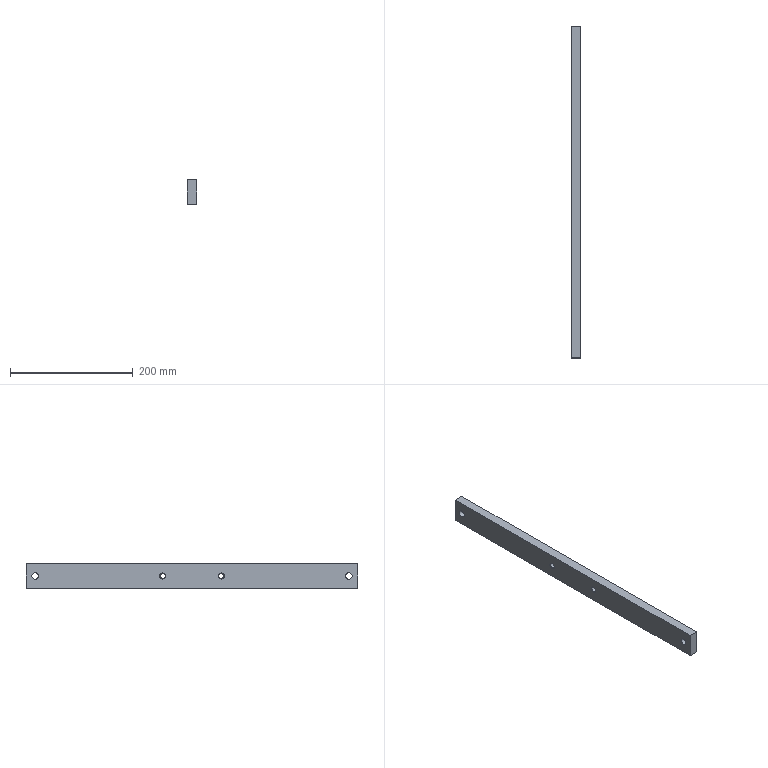Part | STEP file | 冲床-300配套压波_id994_x_t | 1 solid | 14 faces | box 15 x 540 x 40 mm | volume 319568 mm3 | plane 6 | cylinder 4 | cone 4 | commonest cylinder face diameters 8.5 x2 10.7 x2
STEP:
#1=CARTESIAN_POINT('',(1935.,-270.,-185.));
#2=VERTEX_POINT('',#1);
#3=CARTESIAN_POINT('',(1935.,-270.,-225.));
#4=VERTEX_POINT('',#3);
#5=CARTESIAN_POINT('',(1935.,-270.,-185.));
#6=DIRECTION('',(0.,0.,-1.));
#7=VECTOR('',#6,1.);
#8=LINE('',#5,#7);
#9=EDGE_CURVE('',#2,#4,#8,.T.);
#10=ORIENTED_EDGE('',*,*,#9,.F.);
#11=CARTESIAN_POINT('',(1920.,-270.,-185.));
#12=VERTEX_POINT('',#11);
#13=CARTESIAN_POINT('',(1920.,-270.,-185.));
#14=DIRECTION('',(1.,0.,0.));
#15=VECTOR('',#14,1.);
#16=LINE('',#13,#15);
#17=EDGE_CURVE('',#12,#2,#16,.T.);
#18=ORIENTED_EDGE('',*,*,#17,.F.);
#19=CARTESIAN_POINT('',(1920.,-270.,-225.));
#20=VERTEX_POINT('',#19);
#21=CARTESIAN_POINT('',(1920.,-270.,-185.));
#22=DIRECTION('',(0.,0.,-1.));
#23=VECTOR('',#22,1.);
#24=LINE('',#21,#23);
#25=EDGE_CURVE('',#12,#20,#24,.T.);
#26=ORIENTED_EDGE('',*,*,#25,.T.);
#27=CARTESIAN_POINT('',(1920.,-270.,-225.));
#28=DIRECTION('',(1.,0.,0.));
#29=VECTOR('',#28,1.);
#30=LINE('',#27,#29);
#31=EDGE_CURVE('',#20,#4,#30,.T.);
#32=ORIENTED_EDGE('',*,*,#31,.T.);
#33=EDGE_LOOP('',(#10,#18,#26,#32));
#34=FACE_OUTER_BOUND('',#33,.T.);
#35=CARTESIAN_POINT('',(1920.,-270.,-185.));
#36=DIRECTION('',(0.,-1.,0.));
#37=DIRECTION('',(0.,0.,-1.));
#38=AXIS2_PLACEMENT_3D('',#35,#36,#37);
#39=PLANE('',#38);
#40=ADVANCED_FACE('',(#34),#39,.T.);
#41=CARTESIAN_POINT('',(1935.,270.,-225.));
#42=VERTEX_POINT('',#41);
#43=CARTESIAN_POINT('',(1935.,-270.,-225.));
#44=DIRECTION('',(0.,1.,0.));
#45=VECTOR('',#44,1.);
#46=LINE('',#43,#45);
#47=EDGE_CURVE('',#4,#42,#46,.T.);
#48=ORIENTED_EDGE('',*,*,#47,.F.);
#49=ORIENTED_EDGE('',*,*,#31,.F.);
#50=CARTESIAN_POINT('',(1920.,270.,-225.));
#51=VERTEX_POINT('',#50);
#52=CARTESIAN_POINT('',(1920.,-270.,-225.));
#53=DIRECTION('',(0.,1.,0.));
#54=VECTOR('',#53,1.);
#55=LINE('',#52,#54);
#56=EDGE_CURVE('',#20,#51,#55,.T.);
#57=ORIENTED_EDGE('',*,*,#56,.T.);
#58=CARTESIAN_POINT('',(1920.,270.,-225.));
#59=DIRECTION('',(1.,0.,0.));
#60=VECTOR('',#59,1.);
#61=LINE('',#58,#60);
#62=EDGE_CURVE('',#51,#42,#61,.T.);
#63=ORIENTED_EDGE('',*,*,#62,.T.);
#64=EDGE_LOOP('',(#48,#49,#57,#63));
#65=FACE_OUTER_BOUND('',#64,.T.);
#66=CARTESIAN_POINT('',(1920.,-270.,-225.));
#67=DIRECTION('',(0.,0.,-1.));
#68=DIRECTION('',(0.,1.,0.));
#69=AXIS2_PLACEMENT_3D('',#66,#67,#68);
#70=PLANE('',#69);
#71=ADVANCED_FACE('',(#65),#70,.T.);
#72=CARTESIAN_POINT('',(1935.,270.,-185.));
#73=VERTEX_POINT('',#72);
#74=CARTESIAN_POINT('',(1935.,270.,-225.));
#75=DIRECTION('',(0.,0.,1.));
#76=VECTOR('',#75,1.);
#77=LINE('',#74,#76);
#78=EDGE_CURVE('',#42,#73,#77,.T.);
#79=ORIENTED_EDGE('',*,*,#78,.F.);
#80=ORIENTED_EDGE('',*,*,#62,.F.);
#81=CARTESIAN_POINT('',(1920.,270.,-185.));
#82=VERTEX_POINT('',#81);
#83=CARTESIAN_POINT('',(1920.,270.,-225.));
#84=DIRECTION('',(0.,0.,1.));
#85=VECTOR('',#84,1.);
#86=LINE('',#83,#85);
#87=EDGE_CURVE('',#51,#82,#86,.T.);
#88=ORIENTED_EDGE('',*,*,#87,.T.);
#89=CARTESIAN_POINT('',(1920.,270.,-185.));
#90=DIRECTION('',(1.,0.,0.));
#91=VECTOR('',#90,1.);
#92=LINE('',#89,#91);
#93=EDGE_CURVE('',#82,#73,#92,.T.);
#94=ORIENTED_EDGE('',*,*,#93,.T.);
#95=EDGE_LOOP('',(#79,#80,#88,#94));
#96=FACE_OUTER_BOUND('',#95,.T.);
#97=CARTESIAN_POINT('',(1920.,270.,-225.));
#98=DIRECTION('',(0.,1.,0.));
#99=DIRECTION('',(0.,0.,1.));
#100=AXIS2_PLACEMENT_3D('',#97,#98,#99);
#101=PLANE('',#100);
#102=ADVANCED_FACE('',(#96),#101,.T.);
#103=CARTESIAN_POINT('',(1935.,270.,-185.));
#104=DIRECTION('',(0.,-1.,0.));
#105=VECTOR('',#104,1.);
#106=LINE('',#103,#105);
#107=EDGE_CURVE('',#73,#2,#106,.T.);
#108=ORIENTED_EDGE('',*,*,#107,.F.);
#109=ORIENTED_EDGE('',*,*,#93,.F.);
#110=CARTESIAN_POINT('',(1920.,270.,-185.));
#111=DIRECTION('',(0.,-1.,0.));
#112=VECTOR('',#111,1.);
#113=LINE('',#110,#112);
#114=EDGE_CURVE('',#82,#12,#113,.T.);
#115=ORIENTED_EDGE('',*,*,#114,.T.);
#116=ORIENTED_EDGE('',*,*,#17,.T.);
#117=EDGE_LOOP('',(#108,#109,#115,#116));
#118=FACE_OUTER_BOUND('',#117,.T.);
#119=CARTESIAN_POINT('',(1920.,270.,-185.));
#120=DIRECTION('',(0.,0.,1.));
#121=DIRECTION('',(0.,-1.,0.));
#122=AXIS2_PLACEMENT_3D('',#119,#120,#121);
#123=PLANE('',#122);
#124=ADVANCED_FACE('',(#118),#123,.T.);
#125=CARTESIAN_POINT('',(1920.,-255.,-210.35));
#126=VERTEX_POINT('',#125);
#127=CARTESIAN_POINT('',(1920.,-255.,-205.));
#128=DIRECTION('',(-1.,0.,0.));
#129=DIRECTION('',(0.,0.,-1.));
#130=AXIS2_PLACEMENT_3D('',#127,#128,#129);
#131=CIRCLE('',#130,5.35);
#132=EDGE_CURVE('',#126,#126,#131,.T.);
#133=ORIENTED_EDGE('',*,*,#132,.F.);
#134=EDGE_LOOP('',(#133));
#135=FACE_BOUND('',#134,.T.);
#136=CARTESIAN_POINT('',(1920.,255.,-210.35));
#137=VERTEX_POINT('',#136);
#138=CARTESIAN_POINT('',(1920.,255.,-205.));
#139=DIRECTION('',(-1.,0.,0.));
#140=DIRECTION('',(0.,0.,-1.));
#141=AXIS2_PLACEMENT_3D('',#138,#139,#140);
#142=CIRCLE('',#141,5.35);
#143=EDGE_CURVE('',#137,#137,#142,.T.);
#144=ORIENTED_EDGE('',*,*,#143,.F.);
#145=EDGE_LOOP('',(#144));
#146=FACE_BOUND('',#145,.T.);
#147=CARTESIAN_POINT('',(1920.,47.5,-210.));
#148=VERTEX_POINT('',#147);
#149=CARTESIAN_POINT('',(1920.,47.5,-205.));
#150=DIRECTION('',(1.,0.,0.));
#151=DIRECTION('',(0.,0.,-1.));
#152=AXIS2_PLACEMENT_3D('',#149,#150,#151);
#153=CIRCLE('',#152,5.);
#154=EDGE_CURVE('',#148,#148,#153,.T.);
#155=ORIENTED_EDGE('',*,*,#154,.T.);
#156=EDGE_LOOP('',(#155));
#157=FACE_BOUND('',#156,.T.);
#158=CARTESIAN_POINT('',(1920.,-47.5,-210.));
#159=VERTEX_POINT('',#158);
#160=CARTESIAN_POINT('',(1920.,-47.5,-205.));
#161=DIRECTION('',(1.,0.,0.));
#162=DIRECTION('',(0.,0.,-1.));
#163=AXIS2_PLACEMENT_3D('',#160,#161,#162);
#164=CIRCLE('',#163,5.);
#165=EDGE_CURVE('',#159,#159,#164,.T.);
#166=ORIENTED_EDGE('',*,*,#165,.T.);
#167=EDGE_LOOP('',(#166));
#168=FACE_BOUND('',#167,.T.);
#169=ORIENTED_EDGE('',*,*,#25,.F.);
#170=ORIENTED_EDGE('',*,*,#114,.F.);
#171=ORIENTED_EDGE('',*,*,#87,.F.);
#172=ORIENTED_EDGE('',*,*,#56,.F.);
#173=EDGE_LOOP('',(#169,#170,#171,#172));
#174=FACE_BOUND('',#173,.T.);
#175=CARTESIAN_POINT('',(1920.,0.,15.));
#176=DIRECTION('',(1.,0.,0.));
#177=DIRECTION('',(0.,0.,-1.));
#178=AXIS2_PLACEMENT_3D('',#175,#176,#177);
#179=PLANE('',#178);
#180=ADVANCED_FACE('',(#135,#146,#157,#168,#174),#179,.F.);
#181=CARTESIAN_POINT('',(1935.,-255.,-210.35));
#182=VERTEX_POINT('',#181);
#183=CARTESIAN_POINT('',(1935.,-255.,-205.));
#184=DIRECTION('',(-1.,0.,0.));
#185=DIRECTION('',(0.,0.,-1.));
#186=AXIS2_PLACEMENT_3D('',#183,#184,#185);
#187=CIRCLE('',#186,5.35);
#188=EDGE_CURVE('',#182,#182,#187,.T.);
#189=ORIENTED_EDGE('',*,*,#188,.T.);
#190=EDGE_LOOP('',(#189));
#191=FACE_BOUND('',#190,.T.);
#192=CARTESIAN_POINT('',(1935.,255.,-210.35));
#193=VERTEX_POINT('',#192);
#194=CARTESIAN_POINT('',(1935.,255.,-205.));
#195=DIRECTION('',(-1.,0.,0.));
#196=DIRECTION('',(0.,0.,-1.));
#197=AXIS2_PLACEMENT_3D('',#194,#195,#196);
#198=CIRCLE('',#197,5.35);
#199=EDGE_CURVE('',#193,#193,#198,.T.);
#200=ORIENTED_EDGE('',*,*,#199,.T.);
#201=EDGE_LOOP('',(#200));
#202=FACE_BOUND('',#201,.T.);
#203=CARTESIAN_POINT('',(1935.,47.5,-210.));
#204=VERTEX_POINT('',#203);
#205=CARTESIAN_POINT('',(1935.,47.5,-205.));
#206=DIRECTION('',(-1.,0.,0.));
#207=DIRECTION('',(0.,0.,-1.));
#208=AXIS2_PLACEMENT_3D('',#205,#206,#207);
#209=CIRCLE('',#208,5.);
#210=EDGE_CURVE('',#204,#204,#209,.T.);
#211=ORIENTED_EDGE('',*,*,#210,.T.);
#212=EDGE_LOOP('',(#211));
#213=FACE_BOUND('',#212,.T.);
#214=CARTESIAN_POINT('',(1935.,-47.5,-210.));
#215=VERTEX_POINT('',#214);
#216=CARTESIAN_POINT('',(1935.,-47.5,-205.));
#217=DIRECTION('',(-1.,0.,0.));
#218=DIRECTION('',(0.,0.,-1.));
#219=AXIS2_PLACEMENT_3D('',#216,#217,#218);
#220=CIRCLE('',#219,5.);
#221=EDGE_CURVE('',#215,#215,#220,.T.);
#222=ORIENTED_EDGE('',*,*,#221,.T.);
#223=EDGE_LOOP('',(#222));
#224=FACE_BOUND('',#223,.T.);
#225=ORIENTED_EDGE('',*,*,#9,.T.);
#226=ORIENTED_EDGE('',*,*,#47,.T.);
#227=ORIENTED_EDGE('',*,*,#78,.T.);
#228=ORIENTED_EDGE('',*,*,#107,.T.);
#229=EDGE_LOOP('',(#225,#226,#227,#228));
#230=FACE_BOUND('',#229,.T.);
#231=CARTESIAN_POINT('',(1935.,0.,15.));
#232=DIRECTION('',(1.,0.,0.));
#233=DIRECTION('',(0.,0.,-1.));
#234=AXIS2_PLACEMENT_3D('',#231,#232,#233);
#235=PLANE('',#234);
#236=ADVANCED_FACE('',(#191,#202,#213,#224,#230),#235,.T.);
#237=CARTESIAN_POINT('',(1920.75,-47.5,-209.25));
#238=VERTEX_POINT('',#237);
#239=CARTESIAN_POINT('',(1920.75,-47.5,-205.));
#240=DIRECTION('',(-1.,0.,0.));
#241=DIRECTION('',(0.,0.,-1.));
#242=AXIS2_PLACEMENT_3D('',#239,#240,#241);
#243=CIRCLE('',#242,4.25);
#244=EDGE_CURVE('',#238,#238,#243,.T.);
#245=ORIENTED_EDGE('',*,*,#244,.T.);
#246=EDGE_LOOP('',(#245));
#247=FACE_BOUND('',#246,.T.);
#248=CARTESIAN_POINT('',(1934.25,-47.5,-209.25));
#249=VERTEX_POINT('',#248);
#250=CARTESIAN_POINT('',(1934.25,-47.5,-205.));
#251=DIRECTION('',(1.,0.,0.));
#252=DIRECTION('',(0.,0.,-1.));
#253=AXIS2_PLACEMENT_3D('',#250,#251,#252);
#254=CIRCLE('',#253,4.25);
#255=EDGE_CURVE('',#249,#249,#254,.T.);
#256=ORIENTED_EDGE('',*,*,#255,.T.);
#257=EDGE_LOOP('',(#256));
#258=FACE_BOUND('',#257,.T.);
#259=CARTESIAN_POINT('',(1935.,-47.5,-205.));
#260=DIRECTION('',(-1.,0.,0.));
#261=DIRECTION('',(0.,0.,1.));
#262=AXIS2_PLACEMENT_3D('',#259,#260,#261);
#263=CYLINDRICAL_SURFACE('',#262,4.25);
#264=ADVANCED_FACE('',(#247,#258),#263,.F.);
#265=ORIENTED_EDGE('',*,*,#255,.F.);
#266=EDGE_LOOP('',(#265));
#267=FACE_BOUND('',#266,.T.);
#268=ORIENTED_EDGE('',*,*,#221,.F.);
#269=EDGE_LOOP('',(#268));
#270=FACE_BOUND('',#269,.T.);
#271=CARTESIAN_POINT('',(1935.,-47.5,-205.));
#272=DIRECTION('',(1.,0.,0.));
#273=DIRECTION('',(0.,0.,-1.));
#274=AXIS2_PLACEMENT_3D('',#271,#272,#273);
#275=CONICAL_SURFACE('',#274,5.,45.);
#276=ADVANCED_FACE('',(#267,#270),#275,.F.);
#277=ORIENTED_EDGE('',*,*,#244,.F.);
#278=EDGE_LOOP('',(#277));
#279=FACE_BOUND('',#278,.T.);
#280=ORIENTED_EDGE('',*,*,#165,.F.);
#281=EDGE_LOOP('',(#280));
#282=FACE_BOUND('',#281,.T.);
#283=CARTESIAN_POINT('',(1920.,-47.5,-205.));
#284=DIRECTION('',(-1.,0.,0.));
#285=DIRECTION('',(0.,0.,1.));
#286=AXIS2_PLACEMENT_3D('',#283,#284,#285);
#287=CONICAL_SURFACE('',#286,5.,45.);
#288=ADVANCED_FACE('',(#279,#282),#287,.F.);
#289=CARTESIAN_POINT('',(1920.75,47.5,-209.25));
#290=VERTEX_POINT('',#289);
#291=CARTESIAN_POINT('',(1920.75,47.5,-205.));
#292=DIRECTION('',(-1.,0.,0.));
#293=DIRECTION('',(0.,0.,-1.));
#294=AXIS2_PLACEMENT_3D('',#291,#292,#293);
#295=CIRCLE('',#294,4.25);
#296=EDGE_CURVE('',#290,#290,#295,.T.);
#297=ORIENTED_EDGE('',*,*,#296,.T.);
#298=EDGE_LOOP('',(#297));
#299=FACE_BOUND('',#298,.T.);
#300=CARTESIAN_POINT('',(1934.25,47.5,-209.25));
#301=VERTEX_POINT('',#300);
#302=CARTESIAN_POINT('',(1934.25,47.5,-205.));
#303=DIRECTION('',(1.,0.,0.));
#304=DIRECTION('',(0.,0.,-1.));
#305=AXIS2_PLACEMENT_3D('',#302,#303,#304);
#306=CIRCLE('',#305,4.25);
#307=EDGE_CURVE('',#301,#301,#306,.T.);
#308=ORIENTED_EDGE('',*,*,#307,.T.);
#309=EDGE_LOOP('',(#308));
#310=FACE_BOUND('',#309,.T.);
#311=CARTESIAN_POINT('',(1935.,47.5,-205.));
#312=DIRECTION('',(-1.,0.,0.));
#313=DIRECTION('',(0.,0.,1.));
#314=AXIS2_PLACEMENT_3D('',#311,#312,#313);
#315=CYLINDRICAL_SURFACE('',#314,4.25);
#316=ADVANCED_FACE('',(#299,#310),#315,.F.);
#317=ORIENTED_EDGE('',*,*,#307,.F.);
#318=EDGE_LOOP('',(#317));
#319=FACE_BOUND('',#318,.T.);
#320=ORIENTED_EDGE('',*,*,#210,.F.);
#321=EDGE_LOOP('',(#320));
#322=FACE_BOUND('',#321,.T.);
#323=CARTESIAN_POINT('',(1935.,47.5,-205.));
#324=DIRECTION('',(1.,0.,0.));
#325=DIRECTION('',(0.,0.,-1.));
#326=AXIS2_PLACEMENT_3D('',#323,#324,#325);
#327=CONICAL_SURFACE('',#326,5.,45.);
#328=ADVANCED_FACE('',(#319,#322),#327,.F.);
#329=ORIENTED_EDGE('',*,*,#296,.F.);
#330=EDGE_LOOP('',(#329));
#331=FACE_BOUND('',#330,.T.);
#332=ORIENTED_EDGE('',*,*,#154,.F.);
#333=EDGE_LOOP('',(#332));
#334=FACE_BOUND('',#333,.T.);
#335=CARTESIAN_POINT('',(1920.,47.5,-205.));
#336=DIRECTION('',(-1.,0.,0.));
#337=DIRECTION('',(0.,0.,1.));
#338=AXIS2_PLACEMENT_3D('',#335,#336,#337);
#339=CONICAL_SURFACE('',#338,5.,45.);
#340=ADVANCED_FACE('',(#331,#334),#339,.F.);
#341=ORIENTED_EDGE('',*,*,#199,.F.);
#342=EDGE_LOOP('',(#341));
#343=FACE_BOUND('',#342,.T.);
#344=ORIENTED_EDGE('',*,*,#143,.T.);
#345=EDGE_LOOP('',(#344));
#346=FACE_BOUND('',#345,.T.);
#347=CARTESIAN_POINT('',(2085.,255.,-205.));
#348=DIRECTION('',(-1.,0.,0.));
#349=DIRECTION('',(0.,0.,-1.));
#350=AXIS2_PLACEMENT_3D('',#347,#348,#349);
#351=CYLINDRICAL_SURFACE('',#350,5.35);
#352=ADVANCED_FACE('',(#343,#346),#351,.F.);
#353=ORIENTED_EDGE('',*,*,#188,.F.);
#354=EDGE_LOOP('',(#353));
#355=FACE_BOUND('',#354,.T.);
#356=ORIENTED_EDGE('',*,*,#132,.T.);
#357=EDGE_LOOP('',(#356));
#358=FACE_BOUND('',#357,.T.);
#359=CARTESIAN_POINT('',(2085.,-255.,-205.));
#360=DIRECTION('',(-1.,0.,0.));
#361=DIRECTION('',(0.,0.,-1.));
#362=AXIS2_PLACEMENT_3D('',#359,#360,#361);
#363=CYLINDRICAL_SURFACE('',#362,5.35);
#364=ADVANCED_FACE('',(#355,#358),#363,.F.);
#365=CLOSED_SHELL('',(#40,#71,#102,#124,#180,#236,#264,#276,#288,#316,#328,#340,#352,#364));
#366=MANIFOLD_SOLID_BREP('',#365);
#367=(LENGTH_UNIT()NAMED_UNIT(*)SI_UNIT(.MILLI.,.METRE.));
#368=UNCERTAINTY_MEASURE_WITH_UNIT(LENGTH_MEASURE(0.00002),#367,'','');
#369=(NAMED_UNIT(*)PLANE_ANGLE_UNIT()SI_UNIT($,.RADIAN.));
#370=PLANE_ANGLE_MEASURE_WITH_UNIT(PLANE_ANGLE_MEASURE(0.01745),#369);
#371=DIMENSIONAL_EXPONENTS(0.,0.,0.,0.,0.,0.,0.);
#372=(CONVERSION_BASED_UNIT('DEGREE',#370)NAMED_UNIT(#371)PLANE_ANGLE_UNIT());
#373=(NAMED_UNIT(*)SI_UNIT($,.STERADIAN.)SOLID_ANGLE_UNIT());
#374=(GEOMETRIC_REPRESENTATION_CONTEXT(3)GLOBAL_UNCERTAINTY_ASSIGNED_CONTEXT((#368))GLOBAL_UNIT_ASSIGNED_CONTEXT((#367,#372,#373))REPRESENTATION_CONTEXT('',''));
#375=ADVANCED_BREP_SHAPE_REPRESENTATION('',(#366),#374);